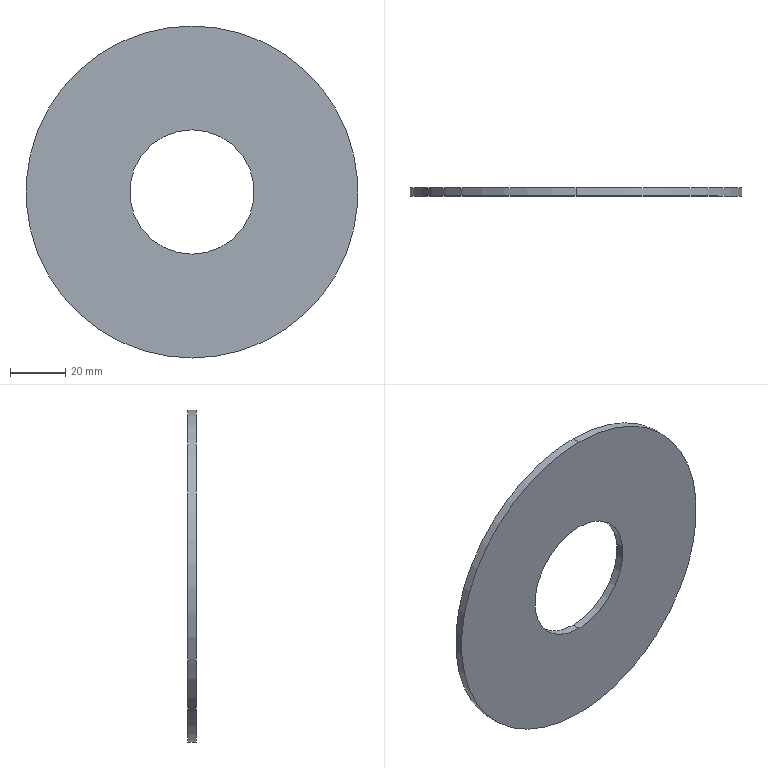Part | SolidWorks | features Extrusion 1 | 1 solid | 6 faces | box 120 x 3 x 120 mm | volume 29158 mm3 | cylinder 4 | plane 2 | commonest cylinder face diameters 45 x2 120 x2
STEP:
#1=CARTESIAN_POINT('',(0.,3.,-22.5));
#2=VERTEX_POINT('',#1);
#3=CARTESIAN_POINT('',(0.,3.,22.5));
#4=VERTEX_POINT('',#3);
#5=CARTESIAN_POINT('',(0.,3.,0.));
#6=DIRECTION('',(0.,1.,0.));
#7=DIRECTION('',(0.,0.,1.));
#8=AXIS2_PLACEMENT_3D('',#5,#6,#7);
#9=CIRCLE('',#8,22.5);
#10=EDGE_CURVE('',#2,#4,#9,.T.);
#11=ORIENTED_EDGE('',*,*,#10,.T.);
#12=CARTESIAN_POINT('',(0.,0.,22.5));
#13=VERTEX_POINT('',#12);
#14=CARTESIAN_POINT('',(0.,3.,22.5));
#15=DIRECTION('',(0.,-1.,0.));
#16=VECTOR('',#15,1000.);
#17=LINE('',#14,#16);
#18=EDGE_CURVE('',#4,#13,#17,.T.);
#19=ORIENTED_EDGE('',*,*,#18,.T.);
#20=CARTESIAN_POINT('',(0.,0.,-22.5));
#21=VERTEX_POINT('',#20);
#22=CARTESIAN_POINT('',(0.,0.,0.));
#23=DIRECTION('',(0.,1.,0.));
#24=DIRECTION('',(0.,0.,1.));
#25=AXIS2_PLACEMENT_3D('',#22,#23,#24);
#26=CIRCLE('',#25,22.5);
#27=EDGE_CURVE('',#21,#13,#26,.T.);
#28=ORIENTED_EDGE('',*,*,#27,.F.);
#29=CARTESIAN_POINT('',(0.,3.,-22.5));
#30=DIRECTION('',(0.,-1.,0.));
#31=VECTOR('',#30,1000.);
#32=LINE('',#29,#31);
#33=EDGE_CURVE('',#2,#21,#32,.T.);
#34=ORIENTED_EDGE('',*,*,#33,.F.);
#35=EDGE_LOOP('',(#11,#19,#28,#34));
#36=FACE_OUTER_BOUND('',#35,.T.);
#37=CARTESIAN_POINT('',(0.,3.,0.));
#38=DIRECTION('',(0.,-1.,0.));
#39=DIRECTION('',(0.,0.,-1.));
#40=AXIS2_PLACEMENT_3D('',#37,#38,#39);
#41=CYLINDRICAL_SURFACE('',#40,22.5);
#42=ADVANCED_FACE('',(#36),#41,.F.);
#43=CARTESIAN_POINT('',(0.,3.,60.));
#44=VERTEX_POINT('',#43);
#45=CARTESIAN_POINT('',(0.,3.,-60.));
#46=VERTEX_POINT('',#45);
#47=CARTESIAN_POINT('',(0.,3.,0.));
#48=DIRECTION('',(0.,1.,0.));
#49=DIRECTION('',(0.,0.,1.));
#50=AXIS2_PLACEMENT_3D('',#47,#48,#49);
#51=CIRCLE('',#50,60.);
#52=EDGE_CURVE('',#44,#46,#51,.T.);
#53=ORIENTED_EDGE('',*,*,#52,.F.);
#54=CARTESIAN_POINT('',(0.,0.,60.));
#55=VERTEX_POINT('',#54);
#56=CARTESIAN_POINT('',(0.,3.,60.));
#57=DIRECTION('',(0.,-1.,0.));
#58=VECTOR('',#57,1000.);
#59=LINE('',#56,#58);
#60=EDGE_CURVE('',#44,#55,#59,.T.);
#61=ORIENTED_EDGE('',*,*,#60,.T.);
#62=CARTESIAN_POINT('',(0.,0.,-60.));
#63=VERTEX_POINT('',#62);
#64=CARTESIAN_POINT('',(0.,0.,0.));
#65=DIRECTION('',(0.,1.,0.));
#66=DIRECTION('',(0.,0.,1.));
#67=AXIS2_PLACEMENT_3D('',#64,#65,#66);
#68=CIRCLE('',#67,60.);
#69=EDGE_CURVE('',#55,#63,#68,.T.);
#70=ORIENTED_EDGE('',*,*,#69,.T.);
#71=CARTESIAN_POINT('',(0.,3.,-60.));
#72=DIRECTION('',(0.,-1.,0.));
#73=VECTOR('',#72,1000.);
#74=LINE('',#71,#73);
#75=EDGE_CURVE('',#46,#63,#74,.T.);
#76=ORIENTED_EDGE('',*,*,#75,.F.);
#77=EDGE_LOOP('',(#53,#61,#70,#76));
#78=FACE_OUTER_BOUND('',#77,.T.);
#79=CARTESIAN_POINT('',(0.,3.,0.));
#80=DIRECTION('',(0.,-1.,0.));
#81=DIRECTION('',(0.,0.,-1.));
#82=AXIS2_PLACEMENT_3D('',#79,#80,#81);
#83=CYLINDRICAL_SURFACE('',#82,60.);
#84=ADVANCED_FACE('',(#78),#83,.T.);
#85=CARTESIAN_POINT('',(0.,3.,0.));
#86=DIRECTION('',(0.,1.,0.));
#87=DIRECTION('',(0.,0.,1.));
#88=AXIS2_PLACEMENT_3D('',#85,#86,#87);
#89=CIRCLE('',#88,60.);
#90=EDGE_CURVE('',#46,#44,#89,.T.);
#91=ORIENTED_EDGE('',*,*,#90,.T.);
#92=ORIENTED_EDGE('',*,*,#52,.T.);
#93=EDGE_LOOP('',(#91,#92));
#94=FACE_OUTER_BOUND('',#93,.T.);
#95=ORIENTED_EDGE('',*,*,#10,.F.);
#96=CARTESIAN_POINT('',(0.,3.,0.));
#97=DIRECTION('',(0.,1.,0.));
#98=DIRECTION('',(0.,0.,1.));
#99=AXIS2_PLACEMENT_3D('',#96,#97,#98);
#100=CIRCLE('',#99,22.5);
#101=EDGE_CURVE('',#4,#2,#100,.T.);
#102=ORIENTED_EDGE('',*,*,#101,.F.);
#103=EDGE_LOOP('',(#95,#102));
#104=FACE_BOUND('',#103,.T.);
#105=CARTESIAN_POINT('',(0.,3.,0.));
#106=DIRECTION('',(0.,1.,0.));
#107=DIRECTION('',(0.,0.,1.));
#108=AXIS2_PLACEMENT_3D('',#105,#106,#107);
#109=PLANE('',#108);
#110=ADVANCED_FACE('',(#94,#104),#109,.T.);
#111=CARTESIAN_POINT('',(0.,0.,0.));
#112=DIRECTION('',(0.,1.,0.));
#113=DIRECTION('',(0.,0.,1.));
#114=AXIS2_PLACEMENT_3D('',#111,#112,#113);
#115=CIRCLE('',#114,60.);
#116=EDGE_CURVE('',#63,#55,#115,.T.);
#117=ORIENTED_EDGE('',*,*,#116,.F.);
#118=ORIENTED_EDGE('',*,*,#69,.F.);
#119=EDGE_LOOP('',(#117,#118));
#120=FACE_OUTER_BOUND('',#119,.T.);
#121=ORIENTED_EDGE('',*,*,#27,.T.);
#122=CARTESIAN_POINT('',(0.,0.,0.));
#123=DIRECTION('',(0.,1.,0.));
#124=DIRECTION('',(0.,0.,1.));
#125=AXIS2_PLACEMENT_3D('',#122,#123,#124);
#126=CIRCLE('',#125,22.5);
#127=EDGE_CURVE('',#13,#21,#126,.T.);
#128=ORIENTED_EDGE('',*,*,#127,.T.);
#129=EDGE_LOOP('',(#121,#128));
#130=FACE_BOUND('',#129,.T.);
#131=CARTESIAN_POINT('',(0.,0.,0.));
#132=DIRECTION('',(0.,1.,0.));
#133=DIRECTION('',(0.,0.,1.));
#134=AXIS2_PLACEMENT_3D('',#131,#132,#133);
#135=PLANE('',#134);
#136=ADVANCED_FACE('',(#120,#130),#135,.F.);
#137=ORIENTED_EDGE('',*,*,#60,.F.);
#138=ORIENTED_EDGE('',*,*,#90,.F.);
#139=ORIENTED_EDGE('',*,*,#75,.T.);
#140=ORIENTED_EDGE('',*,*,#116,.T.);
#141=EDGE_LOOP('',(#137,#138,#139,#140));
#142=FACE_OUTER_BOUND('',#141,.T.);
#143=CARTESIAN_POINT('',(0.,3.,0.));
#144=DIRECTION('',(0.,-1.,0.));
#145=DIRECTION('',(0.,0.,-1.));
#146=AXIS2_PLACEMENT_3D('',#143,#144,#145);
#147=CYLINDRICAL_SURFACE('',#146,60.);
#148=ADVANCED_FACE('',(#142),#147,.T.);
#149=ORIENTED_EDGE('',*,*,#18,.F.);
#150=ORIENTED_EDGE('',*,*,#101,.T.);
#151=ORIENTED_EDGE('',*,*,#33,.T.);
#152=ORIENTED_EDGE('',*,*,#127,.F.);
#153=EDGE_LOOP('',(#149,#150,#151,#152));
#154=FACE_OUTER_BOUND('',#153,.T.);
#155=CARTESIAN_POINT('',(0.,3.,0.));
#156=DIRECTION('',(0.,-1.,0.));
#157=DIRECTION('',(0.,0.,-1.));
#158=AXIS2_PLACEMENT_3D('',#155,#156,#157);
#159=CYLINDRICAL_SURFACE('',#158,22.5);
#160=ADVANCED_FACE('',(#154),#159,.F.);
#161=CLOSED_SHELL('',(#42,#84,#110,#136,#148,#160));
#162=MANIFOLD_SOLID_BREP('',#161);
#163=CARTESIAN_POINT('',(0.,0.,0.));
#164=DIRECTION('',(0.,0.,1.));
#165=DIRECTION('',(1.,0.,0.));
#166=AXIS2_PLACEMENT_3D('',#163,#164,#165);
#167=(LENGTH_UNIT()NAMED_UNIT(*)SI_UNIT(.MILLI.,.METRE.));
#168=UNCERTAINTY_MEASURE_WITH_UNIT(LENGTH_MEASURE(0.00001),#167,'','');
#169=(NAMED_UNIT(*)PLANE_ANGLE_UNIT()SI_UNIT($,.RADIAN.));
#170=(NAMED_UNIT(*)SI_UNIT($,.STERADIAN.)SOLID_ANGLE_UNIT());
#171=(GEOMETRIC_REPRESENTATION_CONTEXT(3)GLOBAL_UNCERTAINTY_ASSIGNED_CONTEXT((#168))GLOBAL_UNIT_ASSIGNED_CONTEXT((#167,#169,#170))REPRESENTATION_CONTEXT('',''));
#172=ADVANCED_BREP_SHAPE_REPRESENTATION('',(#162,#166),#171);